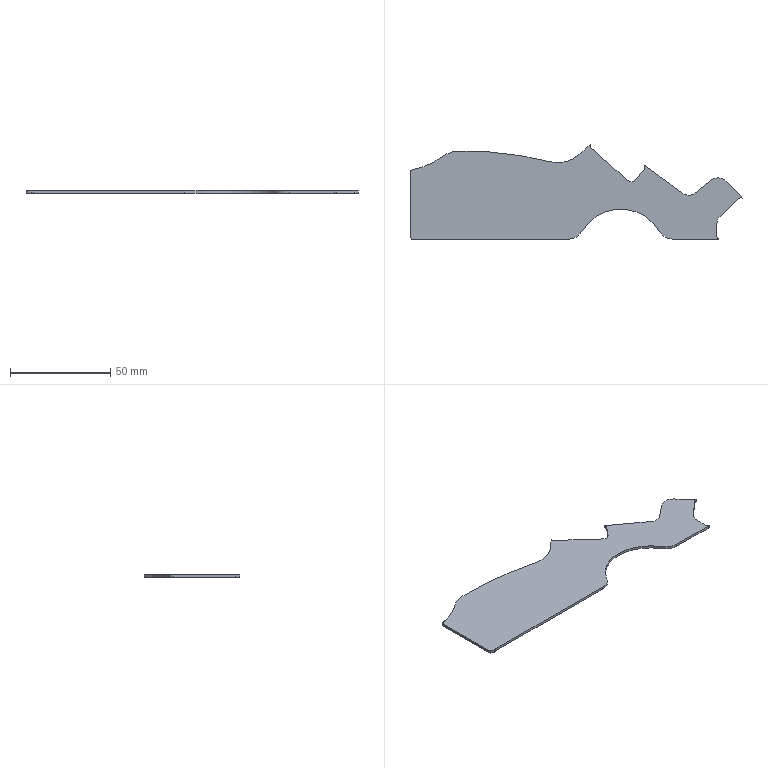Part | STEP file | gslz 2016.10.28-13_id210_x_t | 1 solid | 32 faces | box 165.958 x 47.764 x 1.25 mm | volume 6685 mm3 | cylinder 20 | plane 12 | commonest cylinder face diameters 4 x7 10 x2 16 x2 68.841 x2 6 x1 12 x1